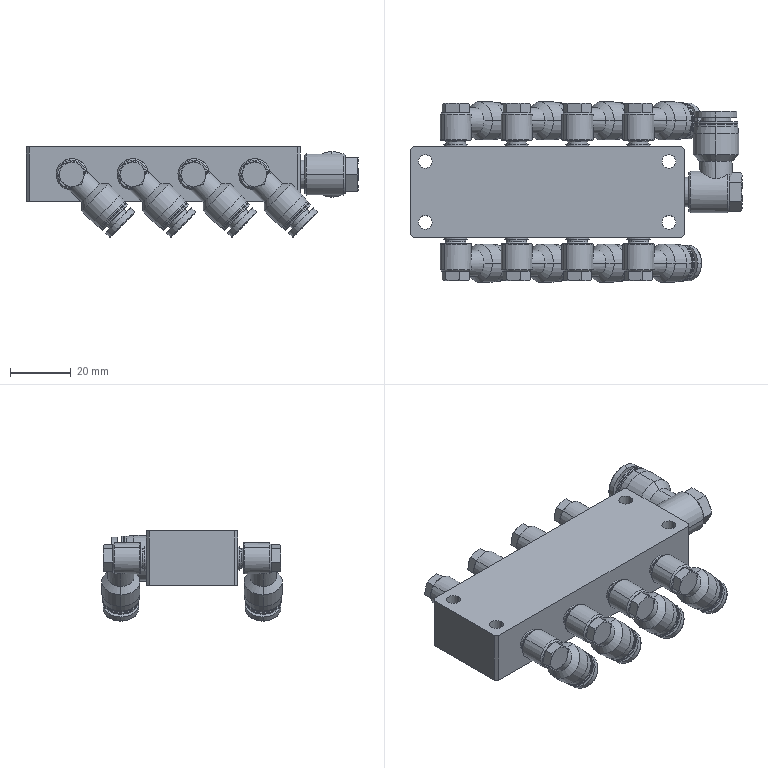Part | SolidWorks | features ReferencePattern 7, DerivedHolePattern 1, MirrorCompFeat 1 | 10 solids | 782 faces | box 109 x 59.2 x 29.612 mm | volume 63942 mm3 | cylinder 289 | plane 230 | cone 184 | spline 79 | commonest cylinder face diameters 11.9 x32 2.5 x16 4 x16 4.2 x16 5 x16 6 x16